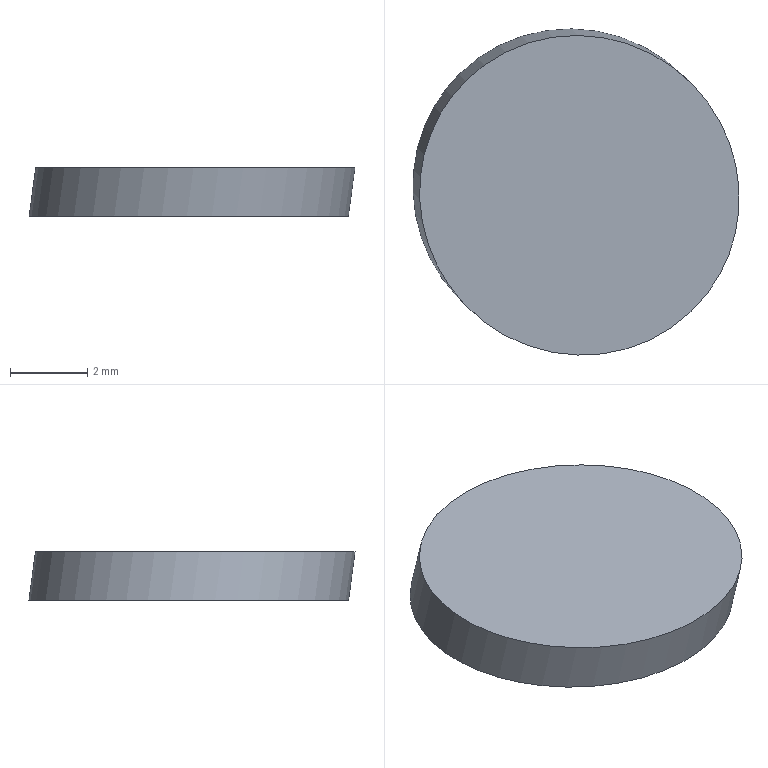Part | STEP file | gslz 2016.10.28-13_id1162_x_t | 1 solid | 3 faces | box 8.449 x 8.449 x 1.25 mm | volume 67.248 mm3 | plane 2 | cylinder 1 | commonest cylinder face diameters 8.2 x1
STEP:
#1=CARTESIAN_POINT('',(0.,0.,0.));
#2=DIRECTION('',(0.,0.,1.));
#3=DIRECTION('',(1.,0.,0.));
#4=AXIS2_PLACEMENT_3D('',#1,#2,#3);
#5=CARTESIAN_POINT('',(992.753,127.688,3.492));
#6=VERTEX_POINT('',#5);
#7=CARTESIAN_POINT('',(995.706,124.735,3.492));
#8=DIRECTION('',(-0.000002457,-0.00000242,-1.));
#9=DIRECTION('',(-0.7071,0.7071,0.000000026));
#10=AXIS2_PLACEMENT_3D('',#7,#8,#9);
#11=ELLIPSE('',#10,4.177,4.1);
#12=CARTESIAN_POINT('',(995.706,124.735,3.492));
#13=DIRECTION('',(0.000002457,0.00000242,1.));
#14=DIRECTION('',(0.7071,0.7071,-0.000003448));
#15=AXIS2_PLACEMENT_3D('',#12,#13,#14);
#16=PLANE('',#15);
#17=CARTESIAN_POINT('',(0.,4.177));
#18=CARTESIAN_POINT('',(7.101,4.177));
#19=CARTESIAN_POINT('',(3.551,-2.088));
#20=CARTESIAN_POINT('',(0.,-8.353));
#21=CARTESIAN_POINT('',(-3.551,-2.088));
#22=CARTESIAN_POINT('',(-7.101,4.177));
#23=CARTESIAN_POINT('',(0.,4.177));
#24=(BOUNDED_CURVE()B_SPLINE_CURVE(2,(#17,#18,#19,#20,#21,#22,#23),.UNSPECIFIED.,.T.,.F.)B_SPLINE_CURVE_WITH_KNOTS((1,2,2,2,2,1),(-2.094,0.,2.094,4.189,6.283,8.378),.UNSPECIFIED.)CURVE()GEOMETRIC_REPRESENTATION_ITEM()RATIONAL_B_SPLINE_CURVE((1.,0.5,1.,0.5,1.,0.5,1.))REPRESENTATION_ITEM(''));
#25=(GEOMETRIC_REPRESENTATION_CONTEXT(2)PARAMETRIC_REPRESENTATION_CONTEXT()REPRESENTATION_CONTEXT('',''));
#26=DEFINITIONAL_REPRESENTATION('',(#24),#25);
#27=PCURVE('',#16,#26);
#28=CARTESIAN_POINT('',(995.706,124.735,3.492));
#29=DIRECTION('',(-0.1349,0.1349,-0.9816));
#30=DIRECTION('',(-0.6941,0.6941,0.1908));
#31=AXIS2_PLACEMENT_3D('',#28,#29,#30);
#32=CYLINDRICAL_SURFACE('',#31,4.1);
#33=CARTESIAN_POINT('',(0.,0.797));
#34=CARTESIAN_POINT('',(0.0952,0.7974));
#35=CARTESIAN_POINT('',(0.2856,0.775));
#36=CARTESIAN_POINT('',(0.5712,0.6797));
#37=CARTESIAN_POINT('',(0.8568,0.529));
#38=CARTESIAN_POINT('',(1.142,0.3356));
#39=CARTESIAN_POINT('',(1.428,0.115));
#40=CARTESIAN_POINT('',(1.714,-0.115));
#41=CARTESIAN_POINT('',(1.999,-0.3356));
#42=CARTESIAN_POINT('',(2.285,-0.529));
#43=CARTESIAN_POINT('',(2.57,-0.6796));
#44=CARTESIAN_POINT('',(2.856,-0.7751));
#45=CARTESIAN_POINT('',(3.142,-0.8079));
#46=CARTESIAN_POINT('',(3.427,-0.7751));
#47=CARTESIAN_POINT('',(3.713,-0.6796));
#48=CARTESIAN_POINT('',(3.998,-0.529));
#49=CARTESIAN_POINT('',(4.284,-0.3356));
#50=CARTESIAN_POINT('',(4.57,-0.115));
#51=CARTESIAN_POINT('',(4.855,0.115));
#52=CARTESIAN_POINT('',(5.141,0.3356));
#53=CARTESIAN_POINT('',(5.426,0.529));
#54=CARTESIAN_POINT('',(5.712,0.6797));
#55=CARTESIAN_POINT('',(5.998,0.775));
#56=CARTESIAN_POINT('',(6.188,0.7974));
#57=CARTESIAN_POINT('',(6.283,0.797));
#58=B_SPLINE_CURVE_WITH_KNOTS('',3,(#33,#34,#35,#36,#37,#38,#39,#40,#41,#42,#43,#44,#45,#46,#47,#48,#49,#50,#51,#52,#53,#54,#55,#56,#57),.UNSPECIFIED.,.F.,.F.,(4,1,1,1,1,1,1,1,1,1,1,1,1,1,1,1,1,1,1,1,1,1,4),(0.,0.2856,0.5712,0.8568,1.142,1.428,1.714,1.999,2.285,2.57,2.856,3.142,3.427,3.713,3.998,4.284,4.57,4.855,5.141,5.426,5.712,5.998,6.283),.QUASI_UNIFORM_KNOTS.);
#59=(GEOMETRIC_REPRESENTATION_CONTEXT(2)PARAMETRIC_REPRESENTATION_CONTEXT()REPRESENTATION_CONTEXT('',''));
#60=DEFINITIONAL_REPRESENTATION('',(#58),#59);
#61=PCURVE('',#32,#60);
#62=SURFACE_CURVE('',#11,(#27,#61),.PCURVE_S1.);
#63=EDGE_CURVE('',#6,#6,#62,.T.);
#64=ORIENTED_EDGE('',*,*,#63,.F.);
#65=EDGE_LOOP('',(#64));
#66=FACE_BOUND('',#65,.T.);
#67=ADVANCED_FACE('',(#66),#16,.T.);
#68=ORIENTED_EDGE('',*,*,#63,.T.);
#69=CARTESIAN_POINT('',(992.581,127.86,2.242));
#70=VERTEX_POINT('',#69);
#71=CARTESIAN_POINT('',(992.753,127.688,3.492));
#72=CARTESIAN_POINT('',(992.581,127.86,2.242));
#73=B_SPLINE_CURVE_WITH_KNOTS('',1,(#71,#72),.UNSPECIFIED.,.F.,.F.,(2,2),(0.797,2.07),.PIECEWISE_BEZIER_KNOTS.);
#74=CARTESIAN_POINT('',(6.283,0.));
#75=DIRECTION('',(0.,1.));
#76=VECTOR('',#75,1.);
#77=LINE('',#74,#76);
#78=(GEOMETRIC_REPRESENTATION_CONTEXT(2)PARAMETRIC_REPRESENTATION_CONTEXT()REPRESENTATION_CONTEXT('',''));
#79=DEFINITIONAL_REPRESENTATION('',(#77),#78);
#80=PCURVE('',#32,#79);
#81=CARTESIAN_POINT('',(0.,0.));
#82=DIRECTION('',(0.,1.));
#83=VECTOR('',#82,1.);
#84=LINE('',#81,#83);
#85=(GEOMETRIC_REPRESENTATION_CONTEXT(2)PARAMETRIC_REPRESENTATION_CONTEXT()REPRESENTATION_CONTEXT('',''));
#86=DEFINITIONAL_REPRESENTATION('',(#84),#85);
#87=PCURVE('',#32,#86);
#88=SEAM_CURVE('',#73,(#80,#87),.PCURVE_S1.);
#89=EDGE_CURVE('',#6,#70,#88,.T.);
#90=ORIENTED_EDGE('',*,*,#89,.T.);
#91=CARTESIAN_POINT('',(995.534,124.907,2.242));
#92=DIRECTION('',(-0.000002457,-0.00000242,-1.));
#93=DIRECTION('',(-0.7071,0.7071,0.000000026));
#94=AXIS2_PLACEMENT_3D('',#91,#92,#93);
#95=ELLIPSE('',#94,4.177,4.1);
#96=CARTESIAN_POINT('',(0.,2.07));
#97=CARTESIAN_POINT('',(0.0952,2.071));
#98=CARTESIAN_POINT('',(0.2856,2.048));
#99=CARTESIAN_POINT('',(0.5712,1.953));
#100=CARTESIAN_POINT('',(0.8568,1.802));
#101=CARTESIAN_POINT('',(1.142,1.609));
#102=CARTESIAN_POINT('',(1.428,1.388));
#103=CARTESIAN_POINT('',(1.714,1.158));
#104=CARTESIAN_POINT('',(1.999,0.9378));
#105=CARTESIAN_POINT('',(2.285,0.7444));
#106=CARTESIAN_POINT('',(2.57,0.5938));
#107=CARTESIAN_POINT('',(2.856,0.4983));
#108=CARTESIAN_POINT('',(3.142,0.4655));
#109=CARTESIAN_POINT('',(3.427,0.4983));
#110=CARTESIAN_POINT('',(3.713,0.5938));
#111=CARTESIAN_POINT('',(3.998,0.7444));
#112=CARTESIAN_POINT('',(4.284,0.9378));
#113=CARTESIAN_POINT('',(4.57,1.158));
#114=CARTESIAN_POINT('',(4.855,1.388));
#115=CARTESIAN_POINT('',(5.141,1.609));
#116=CARTESIAN_POINT('',(5.426,1.802));
#117=CARTESIAN_POINT('',(5.712,1.953));
#118=CARTESIAN_POINT('',(5.998,2.048));
#119=CARTESIAN_POINT('',(6.188,2.071));
#120=CARTESIAN_POINT('',(6.283,2.07));
#121=B_SPLINE_CURVE_WITH_KNOTS('',3,(#96,#97,#98,#99,#100,#101,#102,#103,#104,#105,#106,#107,#108,#109,#110,#111,#112,#113,#114,#115,#116,#117,#118,#119,#120),.UNSPECIFIED.,.F.,.F.,(4,1,1,1,1,1,1,1,1,1,1,1,1,1,1,1,1,1,1,1,1,1,4),(0.,0.2856,0.5712,0.8568,1.142,1.428,1.714,1.999,2.285,2.57,2.856,3.142,3.427,3.713,3.998,4.284,4.57,4.855,5.141,5.426,5.712,5.998,6.283),.QUASI_UNIFORM_KNOTS.);
#122=(GEOMETRIC_REPRESENTATION_CONTEXT(2)PARAMETRIC_REPRESENTATION_CONTEXT()REPRESENTATION_CONTEXT('',''));
#123=DEFINITIONAL_REPRESENTATION('',(#121),#122);
#124=PCURVE('',#32,#123);
#125=CARTESIAN_POINT('',(995.534,124.907,2.242));
#126=DIRECTION('',(0.000002457,0.00000242,1.));
#127=DIRECTION('',(1.,0.,-0.000002457));
#128=AXIS2_PLACEMENT_3D('',#125,#126,#127);
#129=PLANE('',#128);
#130=CARTESIAN_POINT('',(-2.953,2.953));
#131=CARTESIAN_POINT('',(2.068,7.975));
#132=CARTESIAN_POINT('',(3.987,1.034));
#133=CARTESIAN_POINT('',(5.907,-5.907));
#134=CARTESIAN_POINT('',(-1.034,-3.987));
#135=CARTESIAN_POINT('',(-7.975,-2.068));
#136=CARTESIAN_POINT('',(-2.953,2.953));
#137=(BOUNDED_CURVE()B_SPLINE_CURVE(2,(#130,#131,#132,#133,#134,#135,#136),.UNSPECIFIED.,.T.,.F.)B_SPLINE_CURVE_WITH_KNOTS((1,2,2,2,2,1),(-2.094,0.,2.094,4.189,6.283,8.378),.UNSPECIFIED.)CURVE()GEOMETRIC_REPRESENTATION_ITEM()RATIONAL_B_SPLINE_CURVE((1.,0.5,1.,0.5,1.,0.5,1.))REPRESENTATION_ITEM(''));
#138=(GEOMETRIC_REPRESENTATION_CONTEXT(2)PARAMETRIC_REPRESENTATION_CONTEXT()REPRESENTATION_CONTEXT('',''));
#139=DEFINITIONAL_REPRESENTATION('',(#137),#138);
#140=PCURVE('',#129,#139);
#141=SURFACE_CURVE('',#95,(#124,#140),.PCURVE_S1.);
#142=EDGE_CURVE('',#70,#70,#141,.T.);
#143=ORIENTED_EDGE('',*,*,#142,.F.);
#144=ORIENTED_EDGE('',*,*,#89,.F.);
#145=EDGE_LOOP('',(#68,#90,#143,#144));
#146=FACE_BOUND('',#145,.T.);
#147=ADVANCED_FACE('',(#146),#32,.T.);
#148=ORIENTED_EDGE('',*,*,#142,.T.);
#149=EDGE_LOOP('',(#148));
#150=FACE_BOUND('',#149,.T.);
#151=ADVANCED_FACE('',(#150),#129,.F.);
#152=CLOSED_SHELL('',(#67,#147,#151));
#153=MANIFOLD_SOLID_BREP('',#152);
#154=(LENGTH_UNIT()NAMED_UNIT(*)SI_UNIT(.MILLI.,.METRE.));
#155=UNCERTAINTY_MEASURE_WITH_UNIT(LENGTH_MEASURE(0.00001),#154,'','');
#156=(NAMED_UNIT(*)PLANE_ANGLE_UNIT()SI_UNIT($,.RADIAN.));
#157=(NAMED_UNIT(*)SI_UNIT($,.STERADIAN.)SOLID_ANGLE_UNIT());
#158=(GEOMETRIC_REPRESENTATION_CONTEXT(3)GLOBAL_UNCERTAINTY_ASSIGNED_CONTEXT((#155))GLOBAL_UNIT_ASSIGNED_CONTEXT((#154,#156,#157))REPRESENTATION_CONTEXT('',''));
#159=ADVANCED_BREP_SHAPE_REPRESENTATION('',(#4,#153),#158);